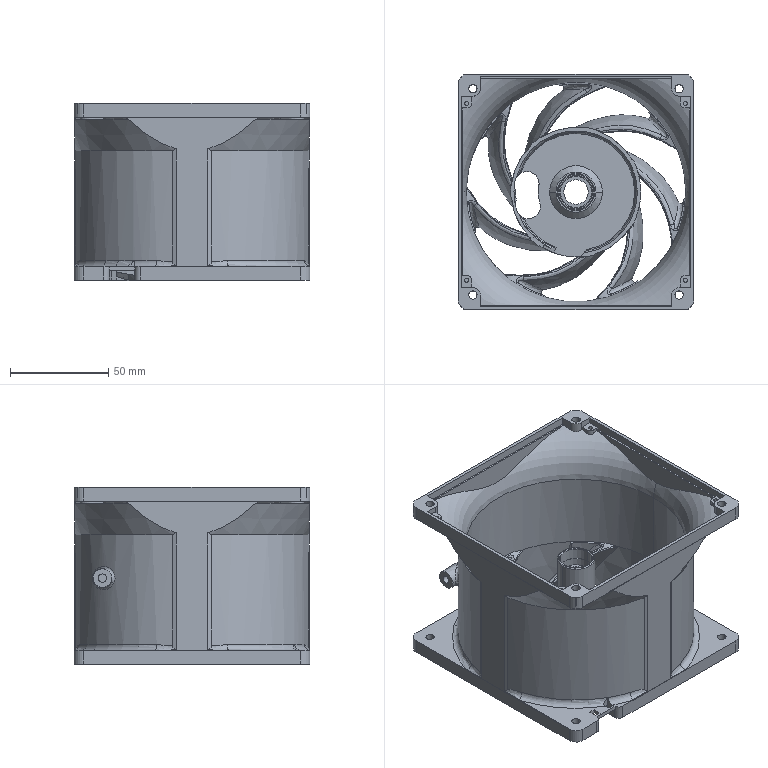NC program | NX | posted with a generic post | part box 120 x 120 x 90.2 mm
Lines 143752 to 144552 of 941997:
(QUICK_ROUGHING_COPY_1 , TOOL : D6-C)
N287442 T04 M6
N287444 G54
N287446 G17 G0 G90 X-31.14 Y23.712 S6800 M3
N287448 G43 Z3.6 H4
N287450 Z-0.4
N287452 G94 G1 Z-0.9 F3000.
N287454 G3 X-27.055 Y23.899 R3.
N287456 G2 X-20.914 Y29.413 R43.89
N287458 X-13.811 Y33.343 R39.638
N287460 X-5.833 Y35.607 R41.306
N287462 X11.068 Y34.326 R36.2
N287464 X16.507 Y32.035 R31.276
N287466 X19.033 Y30.612 R13.271
N287468 X27.771 Y23.006 R34.679
N287470 X33.031 Y14.479 R35.04
N287472 X34.254 Y11.251 R20.013
N287474 X35.286 Y7.405 R25.238
N287476 X36.033 Y-1.242 R34.86
N287478 X33.635 Y-12.989 R34.515
N287480 X28.752 Y-21.784 R34.879
N287482 X26.394 Y-24.597 R40.93
N287484 G1 X24.036 Y-26.923
N287486 G2 X20.106 Y-29.954 R50.066
N287488 X5.172 Y-35.694 R35.887
N287490 X-4.852 Y-35.73 R34.639
N287492 X-13.535 Y-33.468 R36.583
N287494 X-20.751 Y-29.538 R43.309
N287496 G1 X-23.748 Y-27.18
N287498 G2 X-29.413 Y-20.916 R42.927
N287500 G1 X-31.434 Y-17.748
N287502 X-32.557 Y-15.49
N287504 G2 X-34.7 Y-9.888 R34.78
N287506 X-36.039 Y1.968 R38.12
N287508 G1 X-35.622 Y5.833
N287510 X-34.755 Y9.763
N287512 G2 X-31.771 Y17.143 R43.12
N287514 G1 X-29.523 Y20.767
N287516 X-27.055 Y23.899
N287518 G3 X-27.508 Y28.117 R3.
N287520 G1 Z-0.4
N287522 G0 Z0.5
N287524 X-27.506 Y28.118 Z0.552
N287526 X-27.499 Y28.121 Z0.604
N287528 X-27.489 Y28.125 Z0.655
N287530 X-27.474 Y28.131 Z0.705
N287532 X-27.456 Y28.139 Z0.754
N287534 X-27.433 Y28.148 Z0.8
N287536 X-27.407 Y28.159 Z0.844
N287538 X-27.378 Y28.171 Z0.886
N287540 X-27.345 Y28.184 Z0.924
N287542 X-27.31 Y28.199 Z0.96
N287544 X-27.271 Y28.215 Z0.991
N287546 X-27.23 Y28.231 Z1.02
N287548 X-27.187 Y28.249 Z1.044
N287550 X-27.143 Y28.267 Z1.064
N287552 X-27.096 Y28.286 Z1.08
N287554 X-27.049 Y28.306 Z1.091
N287556 X-27.001 Y28.325 Z1.098
N287558 X-26.953 Y28.345 Z1.1
N287560 X-1.252 Y38.897
N287562 X-1.204 Y38.917 Z1.098
N287564 X-1.156 Y38.937 Z1.091
N287566 X-1.109 Y38.956 Z1.08
N287568 X-1.063 Y38.975 Z1.064
N287570 X-1.018 Y38.994 Z1.044
N287572 X-0.975 Y39.011 Z1.02
N287574 X-0.934 Y39.028 Z0.991
N287576 X-0.896 Y39.044 Z0.96
N287578 X-0.86 Y39.059 Z0.924
N287580 X-0.827 Y39.072 Z0.886
N287582 X-0.798 Y39.084 Z0.844
N287584 X-0.772 Y39.095 Z0.8
N287586 X-0.749 Y39.104 Z0.754
N287588 X-0.731 Y39.112 Z0.705
N287590 X-0.716 Y39.118 Z0.655
N287592 X-0.706 Y39.122 Z0.604
N287594 X-0.699 Y39.124 Z0.552
N287596 X-0.697 Y39.125 Z0.5
N287598 Z-0.9
N287600 G1 Z-1.4
N287602 G2 X-3.325 Y35.956 R3.
N287604 X-6.893 Y35.53 R50.606
N287606 G3 X-9.763 Y35.676 R5.3
N287608 X-11.736 Y34.35 R6.44
N287610 G2 X-13.623 Y33.473 R8.727
N287612 G3 X-23.937 Y27.055 R37.614
N287614 X-31.534 Y17.623 R36.833
N287616 G1 X-31.98 Y16.837
N287618 G3 X-33.618 Y15.265 R6.283
N287620 X-34.18 Y12.715 R3.928
N287622 G2 X-34.559 Y10.549 R5.649
N287624 G3 X-35.701 Y5.644 R54.227
N287626 X-36.105 Y1.117 R49.11
N287628 X-34.523 Y-10.674 R37.936
N287630 G1 X-33.095 Y-14.659
N287632 G3 X-32.557 Y-17.546 R4.945
N287634 X-30.76 Y-19.193 R9.859
N287636 G2 X-29.413 Y-21.014 R10.693
N287638 G3 X-23.826 Y-27.18 R43.808
N287640 G1 X-20.767 Y-29.579
N287642 X-16.986 Y-31.896
N287644 X-14.363 Y-33.13
N287646 G2 X-14.161 Y-34.738 R0.96
N287648 G1 X-15.574 Y-35.905
N287650 Z-0.9
N287652 G0 Z0.5
N287654 X-15.572 Y-35.906 Z0.552
N287656 X-15.565 Y-35.908 Z0.604
N287658 X-15.555 Y-35.913 Z0.655
N287660 X-15.54 Y-35.918 Z0.705
N287662 X-15.522 Y-35.926 Z0.754
N287664 X-15.499 Y-35.935 Z0.8
N287666 X-15.473 Y-35.946 Z0.844
N287668 X-15.444 Y-35.958 Z0.886
N287670 X-15.411 Y-35.971 Z0.924
N287672 X-15.375 Y-35.986 Z0.96
N287674 X-15.337 Y-36.001 Z0.991
N287676 X-15.296 Y-36.018 Z1.02
N287678 X-15.253 Y-36.035 Z1.044
N287680 X-15.208 Y-36.054 Z1.064
N287682 X-15.162 Y-36.072 Z1.08
N287684 X-15.114 Y-36.092 Z1.091
N287686 X-15.066 Y-36.111 Z1.098
N287688 X-15.018 Y-36.131 Z1.1
N287690 X-14.504 Y-36.34
N287692 X-14.455 Y-36.36 Z1.098
N287694 X-14.407 Y-36.379 Z1.091
N287696 X-14.36 Y-36.398 Z1.08
N287698 X-14.314 Y-36.417 Z1.064
N287700 X-14.269 Y-36.435 Z1.044
N287702 X-14.226 Y-36.453 Z1.02
N287704 X-14.185 Y-36.47 Z0.991
N287706 X-14.147 Y-36.485 Z0.96
N287708 X-14.111 Y-36.5 Z0.924
N287710 X-14.078 Y-36.513 Z0.886
N287712 X-14.049 Y-36.525 Z0.844
N287714 X-14.023 Y-36.536 Z0.8
N287716 X-14. Y-36.545 Z0.754
N287718 X-13.982 Y-36.552 Z0.705
N287720 X-13.967 Y-36.558 Z0.655
N287722 X-13.957 Y-36.563 Z0.604
N287724 X-13.95 Y-36.565 Z0.552
N287726 X-13.948 Y-36.566 Z0.5
N287728 Z-0.9
N287730 G1 Z-1.4
N287732 G2 X-10.221 Y-34.659 R3.
N287734 X-8.977 Y-35.178 R3.067
N287736 G3 X-6.619 Y-36.387 R5.012
N287738 X-4.379 Y-36.067 R8.899
N287740 G2 X-1.903 Y-36.108 R9.489
N287742 G3 X13.032 Y-33.691 R37.382
N287744 X21.499 Y-29.059 R39.002
N287746 X23.25 Y-28.562 R16.782
N287748 X25.229 Y-26.394 R3.69
N287750 G2 X26.394 Y-24.696 R4.23
N287752 G3 X30.874 Y-18.709 R38.511
N287754 G2 X32.492 Y-18.716 R0.958
N287756 G1 X33.467 Y-20.271
N287758 Z-0.9
N287760 G0 Z0.395
N287762 Z0.413
N287764 X33.469 Y-20.269 Z0.431
N287766 X33.471 Y-20.265 Z0.448
N287768 X33.473 Y-20.261 Z0.465
N287770 X33.477 Y-20.255 Z0.482
N287772 X33.481 Y-20.248 Z0.498
N287774 X33.486 Y-20.24 Z0.513
N287776 X33.492 Y-20.23 Z0.527
N287778 X33.498 Y-20.22 Z0.54
N287780 X33.505 Y-20.209 Z0.552
N287782 X33.512 Y-20.197 Z0.563
N287784 X33.52 Y-20.184 Z0.573
N287786 X33.528 Y-20.17 Z0.581
N287788 X33.537 Y-20.156 Z0.588
N287790 X33.546 Y-20.141 Z0.593
N287792 X33.555 Y-20.127 Z0.597
N287794 X33.564 Y-20.111 Z0.599
N287796 X33.573 Y-20.096 Z0.6
N287798 X33.583 Y-20.081 Z0.599
N287800 X33.592 Y-20.066 Z0.597
N287802 X33.601 Y-20.051 Z0.593
N287804 X33.61 Y-20.036 Z0.588
N287806 X33.618 Y-20.022 Z0.581
N287808 X33.627 Y-20.009 Z0.573
N287810 X33.634 Y-19.996 Z0.563
N287812 X33.642 Y-19.984 Z0.552
N287814 X33.649 Y-19.972 Z0.54
N287816 X33.655 Y-19.962 Z0.527
N287818 X33.661 Y-19.953 Z0.513
N287820 X33.666 Y-19.944 Z0.498
N287822 X33.67 Y-19.937 Z0.482
N287824 X33.673 Y-19.932 Z0.465
N287826 X33.676 Y-19.927 Z0.448
N287828 X33.678 Y-19.924 Z0.431
N287830 X33.679 Y-19.922 Z0.413
N287832 X33.68 Y-19.921 Z0.395
N287834 Z-1.4
N287836 G1 Z-1.9
N287838 X33.671 Y-19.915
N287840 G3 X29.526 Y-20.821 R3.
N287842 G1 X28.355 Y-22.359
N287844 G3 X28.187 Y-23.286 R1.177
N287846 G2 X28.05 Y-25.608 R3.082
N287848 X25.608 Y-28.026 R3.774
N287850 X21.501 Y-29.057 R36.815
N287852 X13.032 Y-33.691 R38.999
N287854 X0.198 Y-36.139 R37.285
N287856 G3 X-0.67 Y-36.612 R1.115
N287858 G2 X-2.689 Y-37.931 R3.404
N287860 X-6.03 Y-37.458 R3.762
N287862 G3 X-7.564 Y-38.185 R1.025
N287864 G1 X-7.827 Y-39.893
N287866 Z-1.4
N287868 G0 Z-0.5
N287870 X-7.825 Y-39.894 Z-0.448
N287872 X-7.819 Y-39.898 Z-0.396
N287874 X-7.809 Y-39.903 Z-0.345
N287876 X-7.795 Y-39.91 Z-0.295
N287878 X-7.777 Y-39.919 Z-0.246
N287880 X-7.755 Y-39.929 Z-0.2
N287882 X-7.73 Y-39.942 Z-0.156
N287884 X-7.702 Y-39.956 Z-0.114
N287886 X-7.67 Y-39.972 Z-0.076
N287888 X-7.636 Y-39.989 Z-0.04
N287890 X-7.598 Y-40.008 Z-0.009
N287892 X-7.559 Y-40.028 Z0.02
N287894 X-7.517 Y-40.048 Z0.044
N287896 X-7.474 Y-40.07 Z0.064
N287898 X-7.43 Y-40.092 Z0.08
N287900 X-7.384 Y-40.115 Z0.091
N287902 X-7.337 Y-40.138 Z0.098
N287904 X-7.291 Y-40.162 Z0.1
N287906 X1.152 Y-44.384
N287908 X1.199 Y-44.407 Z0.098
N287910 X1.245 Y-44.431 Z0.091
N287912 X1.291 Y-44.453 Z0.08
N287914 X1.336 Y-44.476 Z0.064
N287916 X1.379 Y-44.497 Z0.044
N287918 X1.421 Y-44.518 Z0.02
N287920 X1.46 Y-44.538 Z-0.009
N287922 X1.497 Y-44.556 Z-0.04
N287924 X1.532 Y-44.574 Z-0.076
N287926 X1.563 Y-44.59 Z-0.114
N287928 X1.592 Y-44.604 Z-0.156
N287930 X1.617 Y-44.616 Z-0.2
N287932 X1.639 Y-44.627 Z-0.246
N287934 X1.657 Y-44.636 Z-0.295
N287936 X1.671 Y-44.643 Z-0.345
N287938 X1.681 Y-44.648 Z-0.396
N287940 X1.687 Y-44.651 Z-0.448
N287942 X1.689 Y-44.652 Z-0.5
N287944 Z-1.9
N287946 G1 Z-2.4
N287948 G2 X2.731 Y-41.498 R3.
N287950 G3 X4.805 Y-39.071 R6.448
N287952 G2 X5.504 Y-38.71 R1.003
N287954 X8.412 Y-39.409 R4.236
N287956 G1 Z-1.9
N287958 G0 X8.414 Y-39.408 Z-1.856
N287960 X8.419 Y-39.405 Z-1.813
N287962 X8.427 Y-39.401 Z-1.771
N287964 X8.439 Y-39.396 Z-1.729
N287966 X8.454 Y-39.389 Z-1.689
N287968 X8.472 Y-39.38 Z-1.65
N287970 X8.493 Y-39.37 Z-1.613
N287972 X8.517 Y-39.358 Z-1.579
N287974 X8.544 Y-39.346 Z-1.546
N287976 X8.573 Y-39.332 Z-1.517
N287978 X8.604 Y-39.317 Z-1.49
N287980 X8.638 Y-39.301 Z-1.467
N287982 X8.673 Y-39.285 Z-1.447
N287984 X8.709 Y-39.268 Z-1.43
N287986 X8.747 Y-39.25 Z-1.417
N287988 X8.785 Y-39.232 Z-1.408
N287990 X8.824 Y-39.213 Z-1.402
N287992 X8.864 Y-39.194 Z-1.4
N287994 X25.489 Y-31.308
N287996 X25.529 Y-31.289 Z-1.402
N287998 X25.568 Y-31.271 Z-1.408
N288000 X25.606 Y-31.252 Z-1.417
N288002 X25.644 Y-31.234 Z-1.43
N288004 X25.68 Y-31.217 Z-1.447
N288006 X25.715 Y-31.201 Z-1.467
N288008 X25.748 Y-31.185 Z-1.49
N288010 X25.78 Y-31.17 Z-1.517
N288012 X25.809 Y-31.156 Z-1.546
N288014 X25.835 Y-31.144 Z-1.579
N288016 X25.859 Y-31.132 Z-1.613
N288018 X25.88 Y-31.122 Z-1.65
N288020 X25.899 Y-31.114 Z-1.689
N288022 X25.914 Y-31.106 Z-1.729
N288024 X25.926 Y-31.101 Z-1.771
N288026 X25.934 Y-31.097 Z-1.813
N288028 X25.939 Y-31.094 Z-1.856
N288030 X25.941 Y-31.093 Z-1.9
N288032 G1 Z-2.4
N288034 G3 X22.414 Y-28.847 R3.
N288036 X20.824 Y-29.538 R2.587
N288038 G2 X13.032 Y-33.691 R39.322
N288040 X2.857 Y-36.003 R36.76
N288042 G3 X2.329 Y-36.627 R0.68
N288044 G2 X0.456 Y-39.351 R3.019
N288046 X-2.173 Y-39.756 R4.931
N288048 X-3.466 Y-39.244 R4.595
N288050 G3 X-4.964 Y-40.115 R1.056
N288052 G1 X-5.103 Y-41.791
N288054 Z-1.9
N288056 G0 Z-0.627
N288058 X-5.102 Z-0.608
N288060 X-5.1 Y-41.793 Z-0.588
N288062 X-5.096 Y-41.795 Z-0.569
N288064 X-5.091 Y-41.798 Z-0.55
N288066 X-5.085 Y-41.803 Z-0.531
N288068 X-5.077 Y-41.808 Z-0.514
N288070 X-5.068 Y-41.813 Z-0.497
N288072 X-5.058 Y-41.82 Z-0.481
N288074 X-5.047 Y-41.827 Z-0.467
N288076 X-5.034 Y-41.835 Z-0.453
N288078 X-5.021 Y-41.843 Z-0.441
N288080 X-5.007 Y-41.853 Z-0.43
N288082 X-4.992 Y-41.862 Z-0.421
N288084 X-4.977 Y-41.872 Z-0.414
N288086 X-4.961 Y-41.882 Z-0.408
N288088 X-4.945 Y-41.893 Z-0.403
N288090 X-4.928 Y-41.903 Z-0.401
N288092 X-4.912 Y-41.914 Z-0.4
N288094 X-4.895 Y-41.925 Z-0.401
N288096 X-4.878 Y-41.935 Z-0.403
N288098 X-4.862 Y-41.946 Z-0.408
N288100 X-4.846 Y-41.956 Z-0.414
N288102 X-4.831 Y-41.966 Z-0.421
N288104 X-4.816 Y-41.976 Z-0.43
N288106 X-4.802 Y-41.985 Z-0.441
N288108 X-4.789 Y-41.993 Z-0.453
N288110 X-4.776 Y-42.001 Z-0.467
N288112 X-4.765 Y-42.008 Z-0.481
N288114 X-4.755 Y-42.015 Z-0.497
N288116 X-4.746 Y-42.021 Z-0.514
N288118 X-4.738 Y-42.026 Z-0.531
N288120 X-4.732 Y-42.03 Z-0.55
N288122 X-4.727 Y-42.033 Z-0.569
N288124 X-4.723 Y-42.035 Z-0.588
N288126 X-4.721 Y-42.037 Z-0.608
N288128 X-4.72 Z-0.627
N288130 Z-2.4
N288132 G1 Z-2.9
N288134 G2 X-0.848 Y-40.855 R3.
N288136 G3 X2.028 Y-41.242 R3.628
N288138 X3.745 Y-40.542 R6.373
N288140 X4.404 Y-36.374 R3.094
N288142 G2 X4.697 Y-35.803 R0.336
N288144 G3 X20.106 Y-30.006 R35.999
N288146 G2 X21.621 Y-29.012 R16.379
N288148 G1 X22.416 Y-28.847
N288150 G2 X23.613 Y-30.026 R1.01
N288152 G1 X23.283 Y-31.747
N288154 Z-2.4
N288156 G0 Z-1.5
N288158 X23.281 Y-31.748 Z-1.448
N288160 X23.275 Y-31.751 Z-1.396
N288162 X23.265 Y-31.757 Z-1.345
N288164 X23.251 Y-31.764 Z-1.295
N288166 X23.233 Y-31.774 Z-1.246
N288168 X23.212 Y-31.785 Z-1.2
N288170 X23.187 Y-31.798 Z-1.156
N288172 X23.159 Y-31.813 Z-1.114
N288174 X23.128 Y-31.83 Z-1.076
N288176 X23.094 Y-31.848 Z-1.04
N288178 X23.057 Y-31.868 Z-1.009
N288180 X23.018 Y-31.888 Z-0.98
N288182 X22.977 Y-31.91 Z-0.956
N288184 X22.935 Y-31.933 Z-0.936
N288186 X22.891 Y-31.957 Z-0.92
N288188 X22.846 Y-31.981 Z-0.909
N288190 X22.8 Y-32.005 Z-0.902
N288192 X22.754 Y-32.03 Z-0.9
N288194 X15.715 Y-35.789
N288196 X15.669 Y-35.813 Z-0.902
N288198 X15.623 Y-35.838 Z-0.909
N288200 X15.578 Y-35.862 Z-0.92
N288202 X15.534 Y-35.885 Z-0.936
N288204 X15.491 Y-35.908 Z-0.956
N288206 X15.45 Y-35.93 Z-0.98
N288208 X15.411 Y-35.951 Z-1.009
N288210 X15.375 Y-35.97 Z-1.04
N288212 X15.341 Y-35.989 Z-1.076
N288214 X15.31 Y-36.005 Z-1.114
N288216 X15.281 Y-36.02 Z-1.156
N288218 X15.257 Y-36.034 Z-1.2
N288220 X15.235 Y-36.045 Z-1.246
N288222 X15.218 Y-36.054 Z-1.295
N288224 X15.204 Y-36.062 Z-1.345
N288226 X15.194 Y-36.067 Z-1.396
N288228 X15.188 Y-36.07 Z-1.448
N288230 X15.186 Y-36.071 Z-1.5
N288232 Z-2.9
N288234 G1 Z-3.4
N288236 X13.666 Y-36.063
N288238 G3 X10.65 Y-39.046 R3.
N288240 G2 X8.548 Y-44.116 R6.066
N288242 G3 X8.566 Y-46.187 R1.434
N288244 G1 X9.412 Y-46.984
N288246 G2 X9.705 Y-47.665 R0.664
N288248 X8.593 Y-48.068 R1.484
N288250 X-0.276 Y-46.163 R19.273
N288252 X-1.678 Y-44.832 R2.923
N288254 X-1.573 Y-43.936 R1.103
N288256 X2.108 Y-42.464 R3.
N288258 G3 X5.172 Y-42.556 R3.859
N288260 X7.703 Y-39.756 R3.202
N288262 X6.744 Y-37.303 R3.313
N288264 X4.786 Y-36.004 R16.635
N288266 G2 X4.866 Y-35.8 R0.112
N288268 G3 X13.032 Y-33.691 R37.745
N288270 X21.503 Y-29.057 R39.047
N288272 G1 X22.418 Y-28.846
N288274 G2 X23.615 Y-30.026 R1.01
N288276 G1 X23.285 Y-31.747
N288278 Z-2.9
N288280 G0 Z-2.
N288282 X23.287 Y-31.746 Z-1.948
N288284 X23.294 Y-31.745 Z-1.896
N288286 X23.305 Y-31.742 Z-1.845
N288288 X23.32 Y-31.738 Z-1.795
N288290 X23.339 Y-31.733 Z-1.746
N288292 X23.363 Y-31.728 Z-1.7
N288294 X23.39 Y-31.721 Z-1.656
N288296 X23.421 Y-31.713 Z-1.614
N288298 X23.455 Y-31.705 Z-1.576
N288300 X23.493 Y-31.696 Z-1.54
N288302 X23.533 Y-31.686 Z-1.509
N288304 X23.576 Y-31.675 Z-1.48
N288306 X23.621 Y-31.664 Z-1.456
N288308 X23.668 Y-31.653 Z-1.436
N288310 X23.717 Y-31.641 Z-1.42
N288312 X23.766 Y-31.628 Z-1.409
N288314 X23.817 Y-31.616 Z-1.402
N288316 X23.868 Y-31.604 Z-1.4
N288318 X25.365 Y-31.236
N288320 X25.415 Y-31.223 Z-1.402
N288322 X25.466 Y-31.211 Z-1.409
N288324 X25.515 Y-31.199 Z-1.42
N288326 X25.564 Y-31.187 Z-1.436
N288328 X25.611 Y-31.175 Z-1.456
N288330 X25.656 Y-31.164 Z-1.48
N288332 X25.699 Y-31.154 Z-1.509
N288334 X25.739 Y-31.144 Z-1.54
N288336 X25.777 Y-31.135 Z-1.576
N288338 X25.811 Y-31.126 Z-1.614
N288340 X25.842 Y-31.119 Z-1.656
N288342 X25.869 Y-31.112 Z-1.7
N288344 X25.893 Y-31.106 Z-1.746
N288346 X25.912 Y-31.101 Z-1.795
N288348 X25.927 Y-31.098 Z-1.845
N288350 X25.938 Y-31.095 Z-1.896
N288352 X25.945 Y-31.093 Z-1.948
N288354 X25.947 Z-2.
N288356 Z-3.4
N288358 G1 Z-3.9
N288360 G3 X22.42 Y-28.846 R3.
N288362 X20.824 Y-29.538 R2.601
N288364 G2 X13.032 Y-33.691 R39.326
N288366 X5.245 Y-35.755 R38.922
N288368 G3 X5.066 Y-35.924 R0.166
N288370 X5.468 Y-36.226 R0.653
N288372 G1 X8.316 Y-37.745
N288374 G2 X10.408 Y-39.756 R3.81
N288376 X8.503 Y-43.686 R3.028
N288378 X6.744 Y-44.147 R6.29
N288380 X5.253 Y-43.916 R3.933
N288382 G3 X3.923 Y-45.043 R1.066
N288384 G1 X4.073 Y-46.704
N288386 Z-3.4
N288388 G0 Z-2.5
N288390 X4.075 Y-46.705 Z-2.448
N288392 X4.081 Y-46.709 Z-2.396
N288394 X4.09 Y-46.714 Z-2.345
N288396 X4.104 Y-46.723 Z-2.295
N288398 X4.121 Y-46.733 Z-2.246
N288400 X4.142 Y-46.746 Z-2.2
N288402 X4.166 Y-46.76 Z-2.156
N288404 X4.193 Y-46.777 Z-2.114
N288406 X4.223 Y-46.795 Z-2.076
N288408 X4.256 Y-46.815 Z-2.04
N288410 X4.292 Y-46.837 Z-2.009
N288412 X4.329 Y-46.859 Z-1.98
N288414 X4.369 Y-46.884 Z-1.956
N288416 X4.41 Y-46.909 Z-1.936
N288418 X4.453 Y-46.934 Z-1.92
N288420 X4.497 Y-46.961 Z-1.909
N288422 X4.541 Y-46.988 Z-1.902
N288424 X4.586 Y-47.015 Z-1.9
N288426 X6.871 Y-48.401
N288428 X6.916 Y-48.428 Z-1.902
N288430 X6.96 Y-48.455 Z-1.909
N288432 X7.004 Y-48.482 Z-1.92
N288434 X7.047 Y-48.508 Z-1.936
N288436 X7.088 Y-48.533 Z-1.956
N288438 X7.128 Y-48.557 Z-1.98
N288440 X7.165 Y-48.58 Z-2.009
N288442 X7.201 Y-48.601 Z-2.04
N288444 X7.234 Y-48.621 Z-2.076
N288446 X7.264 Y-48.64 Z-2.114
N288448 X7.291 Y-48.656 Z-2.156
N288450 X7.315 Y-48.671 Z-2.2
N288452 X7.336 Y-48.683 Z-2.246
N288454 X7.353 Y-48.694 Z-2.295
N288456 X7.367 Y-48.702 Z-2.345
N288458 X7.376 Y-48.708 Z-2.396
N288460 X7.382 Y-48.711 Z-2.448
N288462 X7.384 Y-48.712 Z-2.5
N288464 Z-3.9
N288466 G1 Z-4.4
N288468 G3 X11.785 Y-47.853 R32.434
N288470 X15.904 Y-44.673 R6.905
N288472 X16.458 Y-40.773 R5.949
N288474 G2 X18.359 Y-38.459 R1.983
N288476 G3 X25.345 Y-34.228 R10.358
N288478 X25.949 Y-31.093 R3.772
N288480 X22.422 Y-28.845 R3.
N288482 X20.824 Y-29.538 R2.606
N288484 G2 X13.032 Y-33.691 R39.327
N288486 X5.615 Y-35.695 R38.961
N288488 G3 X5.321 Y-35.873 R0.246
N288490 X5.724 Y-36.179 R0.635
N288492 X11.569 Y-38.97 R49.433
N288494 G2 X13.296 Y-40.542 R3.833
N288496 X11.46 Y-44.799 R3.075
N288498 X8.975 Y-45.258 R4.65
N288500 X7.85 Y-44.97 R5.548
N288502 G3 X6.448 Y-46.022 R1.073
N288504 G1 X6.496 Y-47.688
N288506 Z-3.9
N288508 G0 Z-2.5
N288510 X6.497 Y-47.69 Z-2.448
N288512 X6.501 Y-47.696 Z-2.396
N288514 X6.507 Y-47.705 Z-2.345
N288516 X6.516 Y-47.718 Z-2.295
N288518 X6.527 Y-47.735 Z-2.246
N288520 X6.54 Y-47.755 Z-2.2
N288522 X6.556 Y-47.779 Z-2.156
N288524 X6.573 Y-47.805 Z-2.114
N288526 X6.593 Y-47.835 Z-2.076
N288528 X6.614 Y-47.867 Z-2.04
N288530 X6.637 Y-47.901 Z-2.009
N288532 X6.661 Y-47.938 Z-1.98
N288534 X6.687 Y-47.977 Z-1.956
N288536 X6.714 Y-48.017 Z-1.936
N288538 X6.741 Y-48.059 Z-1.92
N288540 X6.769 Y-48.102 Z-1.909
N288542 X6.798 Y-48.145 Z-1.902
N288544 X6.827 Y-48.188 Z-1.9
N288546 X7.063 Y-48.546
N288548 X7.092 Y-48.59 Z-1.902
N288550 X7.121 Y-48.633 Z-1.909
N288552 X7.149 Y-48.676 Z-1.92
N288554 X7.177 Y-48.717 Z-1.936
N288556 X7.203 Y-48.758 Z-1.956
N288558 X7.229 Y-48.796 Z-1.98
N288560 X7.253 Y-48.833 Z-2.009
N288562 X7.276 Y-48.868 Z-2.04
N288564 X7.297 Y-48.9 Z-2.076
N288566 X7.317 Y-48.93 Z-2.114
N288568 X7.335 Y-48.956 Z-2.156
N288570 X7.35 Y-48.98 Z-2.2
N288572 X7.363 Y-49. Z-2.246
N288574 X7.374 Y-49.016 Z-2.295
N288576 X7.383 Y-49.03 Z-2.345
N288578 X7.389 Y-49.039 Z-2.396
N288580 X7.393 Y-49.045 Z-2.448
N288582 X7.394 Y-49.047 Z-2.5
N288584 Z-3.9
N288586 G1 Z-4.4
N288588 G3 X10.364 Y-49.441 R4.351
N288590 X18.365 Y-47.083 R49.521
N288592 X20.635 Y-45.13 R4.765
N288594 G2 X23.687 Y-43.753 R3.59
N288596 X24.425 Y-44.257 R1.012
N288598 G1 X24.44 Y-44.287
N288600 G2 X23.111 Y-48.316 R3.
N288602 X8.517 Y-52.876 R53.857
N288604 G1 X7.336 Y-53.026
N288606 G2 X6.159 Y-51.736 R1.068
N288608 G1 X6.518 Y-50.105
N288610 Z-3.9
N288612 G0 Z-3.
N288614 X6.52 Y-50.103 Z-2.948
N288616 X6.524 Y-50.098 Z-2.896
N288618 X6.53 Y-50.089 Z-2.845
N288620 X6.54 Y-50.076 Z-2.795
N288622 X6.551 Y-50.06 Z-2.746
N288624 X6.566 Y-50.04 Z-2.7
N288626 X6.582 Y-50.017 Z-2.656
N288628 X6.601 Y-49.992 Z-2.614
N288630 X6.622 Y-49.963 Z-2.576
N288632 X6.644 Y-49.932 Z-2.54
N288634 X6.669 Y-49.898 Z-2.509
N288636 X6.695 Y-49.862 Z-2.48
N288638 X6.722 Y-49.825 Z-2.456
N288640 X6.75 Y-49.786 Z-2.436
N288642 X6.78 Y-49.745 Z-2.42
N288644 X6.81 Y-49.704 Z-2.409
N288646 X6.84 Y-49.662 Z-2.402
N288648 X6.871 Y-49.62 Z-2.4
N288650 X7.042 Y-49.383
N288652 X7.073 Y-49.341 Z-2.402
N288654 X7.103 Y-49.299 Z-2.409
N288656 X7.133 Y-49.258 Z-2.42
N288658 X7.162 Y-49.217 Z-2.436
N288660 X7.191 Y-49.178 Z-2.456
N288662 X7.218 Y-49.141 Z-2.48
N288664 X7.244 Y-49.105 Z-2.509
N288666 X7.268 Y-49.071 Z-2.54
N288668 X7.291 Y-49.04 Z-2.576
N288670 X7.312 Y-49.011 Z-2.614
N288672 X7.331 Y-48.986 Z-2.656
N288674 X7.347 Y-48.963 Z-2.7
N288676 X7.361 Y-48.943 Z-2.746
N288678 X7.373 Y-48.927 Z-2.795
N288680 X7.382 Y-48.914 Z-2.845
N288682 X7.389 Y-48.905 Z-2.896
N288684 X7.393 Y-48.9 Z-2.948
N288686 X7.394 Y-48.898 Z-3.
N288688 Z-4.4
N288690 G1 Z-4.9
N288692 G3 X10.346 Y-49.427 R3.878
N288694 X11.406 Y-49.154 R4.453
N288696 G1 X10.392 Y-48.934
N288698 G3 X7.394 Y-48.898 R5.735
N288700 G1 Z-4.4
N288702 G0 Z-3.
N288704 X7.396 Y-48.897 Z-2.948
N288706 X7.403 Y-48.895 Z-2.896
N288708 X7.414 Y-48.892 Z-2.845
N288710 X7.429 Y-48.887 Z-2.795
N288712 X7.448 Y-48.882 Z-2.746
N288714 X7.471 Y-48.875 Z-2.7
N288716 X7.498 Y-48.867 Z-2.656
N288718 X7.529 Y-48.858 Z-2.614
N288720 X7.563 Y-48.848 Z-2.576
N288722 X7.6 Y-48.837 Z-2.54
N288724 X7.64 Y-48.826 Z-2.509
N288726 X7.682 Y-48.813 Z-2.48
N288728 X7.727 Y-48.8 Z-2.456
N288730 X7.773 Y-48.786 Z-2.436
N288732 X7.821 Y-48.772 Z-2.42
N288734 X7.87 Y-48.758 Z-2.409
N288736 X7.92 Y-48.743 Z-2.402
N288738 X7.97 Y-48.729 Z-2.4
N288740 X20.552 Y-45.032
N288742 Z-4.4
N288744 G1 Z-4.9
N288746 X18.145 Y-46.825
N288748 X17.589 Y-47.383
N288750 X18.354 Y-47.068
N288752 G3 X20.622 Y-45.114 R4.761
N288754 G1 Z-4.4
N288756 G0 Z-3.
N288758 X20.625 Y-45.113 Z-2.948
N288760 X20.631 Y-45.112 Z-2.896
N288762 X20.642 Y-45.109 Z-2.845
N288764 X20.658 Y-45.105 Z-2.795
N288766 X20.677 Y-45.1 Z-2.746
N288768 X20.7 Y-45.094 Z-2.7
N288770 X20.728 Y-45.088 Z-2.656
N288772 X20.759 Y-45.08 Z-2.614
N288774 X20.793 Y-45.071 Z-2.576
N288776 X20.83 Y-45.062 Z-2.54
N288778 X20.871 Y-45.052 Z-2.509
N288780 X20.914 Y-45.041 Z-2.48
N288782 X20.959 Y-45.03 Z-2.456
N288784 X21.005 Y-45.018 Z-2.436
N288786 X21.054 Y-45.006 Z-2.42
N288788 X21.103 Y-44.994 Z-2.409
N288790 X21.154 Y-44.981 Z-2.402
N288792 X21.205 Y-44.968 Z-2.4
N288794 X24.627 Y-44.114
N288796 Z-4.4
N288798 G1 Z-4.9
N288800 X24.653 Y-44.164
N288802 G2 X23.321 Y-48.192 R3.
N288804 X7.366 Y-53.005 R52.47
N288806 X6.136 Y-51.704 R1.108
N288808 G1 X6.428 Y-50.119
N288810 Z-4.4
N288812 G0 Z-3.
N288814 X6.426 Y-50.117 Z-2.948
N288816 X6.422 Y-50.112 Z-2.896
N288818 X6.416 Y-50.102 Z-2.845
N288820 X6.407 Y-50.089 Z-2.795
N288822 X6.396 Y-50.073 Z-2.746
N288824 X6.382 Y-50.053 Z-2.7
N288826 X6.366 Y-50.03 Z-2.656
N288828 X6.348 Y-50.003 Z-2.614
N288830 X6.328 Y-49.974 Z-2.576
N288832 X6.306 Y-49.942 Z-2.54
N288834 X6.283 Y-49.908 Z-2.509
N288836 X6.258 Y-49.872 Z-2.48
N288838 X6.231 Y-49.834 Z-2.456
N288840 X6.204 Y-49.794 Z-2.436
N288842 X6.176 Y-49.753 Z-2.42
N288844 X6.147 Y-49.71 Z-2.409
N288846 X6.118 Y-49.668 Z-2.402
N288848 X6.088 Y-49.625 Z-2.4
N288850 X4.433 Y-47.216
N288852 X4.404 Y-47.173 Z-2.402
N288854 X4.374 Y-47.13 Z-2.409
N288856 X4.345 Y-47.088 Z-2.42
N288858 X4.317 Y-47.047 Z-2.436
N288860 X4.29 Y-47.007 Z-2.456
N288862 X4.264 Y-46.969 Z-2.48
N288864 X4.239 Y-46.933 Z-2.509
N288866 X4.215 Y-46.898 Z-2.54
N288868 X4.193 Y-46.867 Z-2.576
N288870 X4.173 Y-46.838 Z-2.614
N288872 X4.155 Y-46.811 Z-2.656
N288874 X4.139 Y-46.788 Z-2.7
N288876 X4.125 Y-46.768 Z-2.746
N288878 X4.114 Y-46.752 Z-2.795
N288880 X4.105 Y-46.739 Z-2.845
N288882 X4.099 Y-46.729 Z-2.896
N288884 X4.095 Y-46.724 Z-2.948
N288886 X4.094 Y-46.722 Z-3.
N288888 Z-4.4
N288890 G1 Z-4.9
N288892 G2 X7.876 Y-44.988 R3.
N288894 G3 X12.246 Y-46.242 R21.159
N288896 X14.604 Y-45.691 R4.599
N288898 X16.699 Y-42.114 R3.118
N288900 X14.604 Y-39.832 R3.364
N288902 G2 X5.715 Y-35.966 R44.908
N288904 X5.768 Y-35.7 R0.141
N288906 G1 X9.888 Y-34.761
N288908 X13.032 Y-33.691
N288910 G3 X17.748 Y-31.459 R40.304
N288912 X21.58 Y-29.025 R59.814
N288914 G1 X22.424 Y-28.845
N288916 G2 X23.621 Y-30.025 R1.01
N288918 G1 X23.291 Y-31.746
N288920 Z-4.4
N288922 G0 Z-3.5
N288924 Y-31.748 Z-3.448
N288926 Y-31.755 Z-3.396
N288928 Y-31.766 Z-3.345
N288930 Y-31.782 Z-3.295
N288932 Y-31.802 Z-3.246
N288934 Y-31.826 Z-3.2
N288936 Y-31.854 Z-3.156
N288938 Y-31.886 Z-3.114
N288940 Y-31.921 Z-3.076
N288942 Y-31.96 Z-3.04
N288944 Y-32.001 Z-3.009
N288946 Y-32.046 Z-2.98
N288948 Y-32.092 Z-2.956
N288950 Y-32.14 Z-2.936
N288952 Y-32.19 Z-2.92
N288954 Y-32.241 Z-2.909
N288956 Y-32.293 Z-2.902
N288958 X23.292 Y-32.346 Z-2.9
N288960 X23.299 Y-37.753
N288962 Y-37.805 Z-2.902
N288964 Y-37.857 Z-2.909
N288966 Y-37.908 Z-2.92
N288968 Y-37.958 Z-2.936
N288970 Y-38.006 Z-2.956
N288972 Y-38.053 Z-2.98
N288974 Y-38.097 Z-3.009
N288976 Y-38.138 Z-3.04
N288978 Y-38.177 Z-3.076
N288980 Y-38.212 Z-3.114
N288982 Y-38.244 Z-3.156
N288984 Y-38.272 Z-3.2
N288986 X23.3 Y-38.296 Z-3.246
N288988 Y-38.316 Z-3.295
N288990 Y-38.332 Z-3.345
N288992 Y-38.343 Z-3.396
N288994 Y-38.35 Z-3.448
N288996 Y-38.353 Z-3.5
N288998 Z-4.9
N289000 G1 Z-5.4
N289002 G3 X22.627 Y-41.343 R3.
N289004 G2 X22.865 Y-44.67 R6.262
N289006 G3 X23.319 Y-44.797 R0.261
N289008 G1 X24.85 Y-43.986
N289010 G3 X26.858 Y-41.765 R4.848
N289012 G1 Z-4.9
N289014 G0 Z-3.5
N289016 X26.856 Y-41.766 Z-3.448
N289018 X26.849 Y-41.768 Z-3.396
N289020 X26.839 Y-41.772 Z-3.345
N289022 X26.824 Y-41.777 Z-3.295
N289024 X26.805 Y-41.784 Z-3.246
N289026 X26.783 Y-41.792 Z-3.2
N289028 X26.756 Y-41.802 Z-3.156
N289030 X26.726 Y-41.813 Z-3.114
N289032 X26.693 Y-41.825 Z-3.076
N289034 X26.657 Y-41.838 Z-3.04
N289036 X26.618 Y-41.853 Z-3.009